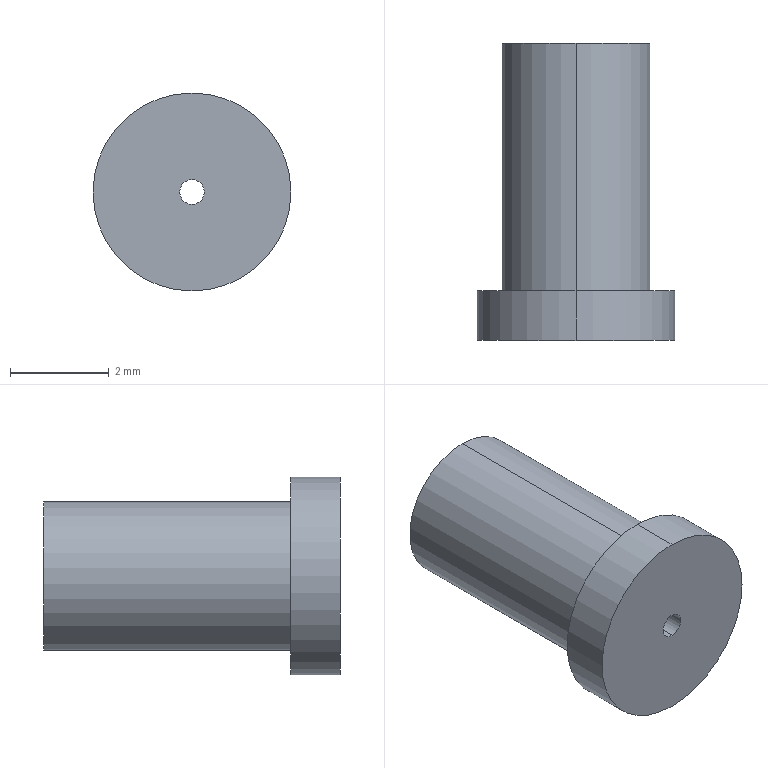Part | SolidWorks | features Revolution 1 | 1 solid | 9 faces | box 4 x 6 x 4 mm | volume 46.731 mm3 | cylinder 6 | plane 3 | commonest cylinder face diameters 0.5 x2 3 x2 4 x2
STEP:
#1=CARTESIAN_POINT('',(0.,3.773,-1.5));
#2=VERTEX_POINT('',#1);
#3=CARTESIAN_POINT('',(0.,3.773,1.5));
#4=VERTEX_POINT('',#3);
#5=CARTESIAN_POINT('',(0.,3.773,0.));
#6=DIRECTION('',(0.,-1.,0.));
#7=DIRECTION('',(0.,0.,-1.));
#8=AXIS2_PLACEMENT_3D('',#5,#6,#7);
#9=CIRCLE('',#8,1.5);
#10=EDGE_CURVE('',#2,#4,#9,.T.);
#11=ORIENTED_EDGE('',*,*,#10,.T.);
#12=CARTESIAN_POINT('',(0.,-1.227,1.5));
#13=VERTEX_POINT('',#12);
#14=CARTESIAN_POINT('',(0.,0.,1.5));
#15=DIRECTION('',(0.,-1.,0.));
#16=VECTOR('',#15,1000.);
#17=LINE('',#14,#16);
#18=EDGE_CURVE('',#4,#13,#17,.T.);
#19=ORIENTED_EDGE('',*,*,#18,.T.);
#20=CARTESIAN_POINT('',(0.,-1.227,-1.5));
#21=VERTEX_POINT('',#20);
#22=CARTESIAN_POINT('',(0.,-1.227,0.));
#23=DIRECTION('',(0.,-1.,0.));
#24=DIRECTION('',(0.,0.,-1.));
#25=AXIS2_PLACEMENT_3D('',#22,#23,#24);
#26=CIRCLE('',#25,1.5);
#27=EDGE_CURVE('',#21,#13,#26,.T.);
#28=ORIENTED_EDGE('',*,*,#27,.F.);
#29=CARTESIAN_POINT('',(0.,0.,-1.5));
#30=DIRECTION('',(0.,-1.,0.));
#31=VECTOR('',#30,1000.);
#32=LINE('',#29,#31);
#33=EDGE_CURVE('',#2,#21,#32,.T.);
#34=ORIENTED_EDGE('',*,*,#33,.F.);
#35=EDGE_LOOP('',(#11,#19,#28,#34));
#36=FACE_OUTER_BOUND('',#35,.T.);
#37=CARTESIAN_POINT('',(0.,0.,0.));
#38=DIRECTION('',(0.,-1.,0.));
#39=DIRECTION('',(0.,0.,-1.));
#40=AXIS2_PLACEMENT_3D('',#37,#38,#39);
#41=CYLINDRICAL_SURFACE('',#40,1.5);
#42=ADVANCED_FACE('',(#36),#41,.T.);
#43=CARTESIAN_POINT('',(0.,-1.227,-2.));
#44=VERTEX_POINT('',#43);
#45=CARTESIAN_POINT('',(0.,-1.227,2.));
#46=VERTEX_POINT('',#45);
#47=CARTESIAN_POINT('',(0.,-1.227,0.));
#48=DIRECTION('',(0.,-1.,0.));
#49=DIRECTION('',(0.,0.,-1.));
#50=AXIS2_PLACEMENT_3D('',#47,#48,#49);
#51=CIRCLE('',#50,2.);
#52=EDGE_CURVE('',#44,#46,#51,.T.);
#53=ORIENTED_EDGE('',*,*,#52,.T.);
#54=CARTESIAN_POINT('',(0.,-2.227,2.));
#55=VERTEX_POINT('',#54);
#56=CARTESIAN_POINT('',(0.,0.,2.));
#57=DIRECTION('',(0.,-1.,0.));
#58=VECTOR('',#57,1000.);
#59=LINE('',#56,#58);
#60=EDGE_CURVE('',#46,#55,#59,.T.);
#61=ORIENTED_EDGE('',*,*,#60,.T.);
#62=CARTESIAN_POINT('',(0.,-2.227,-2.));
#63=VERTEX_POINT('',#62);
#64=CARTESIAN_POINT('',(0.,-2.227,0.));
#65=DIRECTION('',(0.,-1.,0.));
#66=DIRECTION('',(0.,0.,-1.));
#67=AXIS2_PLACEMENT_3D('',#64,#65,#66);
#68=CIRCLE('',#67,2.);
#69=EDGE_CURVE('',#63,#55,#68,.T.);
#70=ORIENTED_EDGE('',*,*,#69,.F.);
#71=CARTESIAN_POINT('',(0.,0.,-2.));
#72=DIRECTION('',(0.,-1.,0.));
#73=VECTOR('',#72,1000.);
#74=LINE('',#71,#73);
#75=EDGE_CURVE('',#44,#63,#74,.T.);
#76=ORIENTED_EDGE('',*,*,#75,.F.);
#77=EDGE_LOOP('',(#53,#61,#70,#76));
#78=FACE_OUTER_BOUND('',#77,.T.);
#79=CARTESIAN_POINT('',(0.,0.,0.));
#80=DIRECTION('',(0.,-1.,0.));
#81=DIRECTION('',(0.,0.,-1.));
#82=AXIS2_PLACEMENT_3D('',#79,#80,#81);
#83=CYLINDRICAL_SURFACE('',#82,2.);
#84=ADVANCED_FACE('',(#78),#83,.T.);
#85=CARTESIAN_POINT('',(0.,3.773,0.25));
#86=VERTEX_POINT('',#85);
#87=CARTESIAN_POINT('',(0.,3.773,-0.25));
#88=VERTEX_POINT('',#87);
#89=CARTESIAN_POINT('',(0.,3.773,0.));
#90=DIRECTION('',(0.,-1.,0.));
#91=DIRECTION('',(0.,0.,-1.));
#92=AXIS2_PLACEMENT_3D('',#89,#90,#91);
#93=CIRCLE('',#92,0.25);
#94=EDGE_CURVE('',#86,#88,#93,.T.);
#95=ORIENTED_EDGE('',*,*,#94,.F.);
#96=CARTESIAN_POINT('',(0.,-2.227,0.25));
#97=VERTEX_POINT('',#96);
#98=CARTESIAN_POINT('',(0.,0.,0.25));
#99=DIRECTION('',(0.,-1.,0.));
#100=VECTOR('',#99,1000.);
#101=LINE('',#98,#100);
#102=EDGE_CURVE('',#86,#97,#101,.T.);
#103=ORIENTED_EDGE('',*,*,#102,.T.);
#104=CARTESIAN_POINT('',(0.,-2.227,-0.25));
#105=VERTEX_POINT('',#104);
#106=CARTESIAN_POINT('',(0.,-2.227,0.));
#107=DIRECTION('',(0.,-1.,0.));
#108=DIRECTION('',(0.,0.,-1.));
#109=AXIS2_PLACEMENT_3D('',#106,#107,#108);
#110=CIRCLE('',#109,0.25);
#111=EDGE_CURVE('',#97,#105,#110,.T.);
#112=ORIENTED_EDGE('',*,*,#111,.T.);
#113=CARTESIAN_POINT('',(0.,0.,-0.25));
#114=DIRECTION('',(0.,-1.,0.));
#115=VECTOR('',#114,1000.);
#116=LINE('',#113,#115);
#117=EDGE_CURVE('',#88,#105,#116,.T.);
#118=ORIENTED_EDGE('',*,*,#117,.F.);
#119=EDGE_LOOP('',(#95,#103,#112,#118));
#120=FACE_OUTER_BOUND('',#119,.T.);
#121=CARTESIAN_POINT('',(0.,0.,0.));
#122=DIRECTION('',(0.,-1.,0.));
#123=DIRECTION('',(0.,0.,-1.));
#124=AXIS2_PLACEMENT_3D('',#121,#122,#123);
#125=CYLINDRICAL_SURFACE('',#124,0.25);
#126=ADVANCED_FACE('',(#120),#125,.F.);
#127=CARTESIAN_POINT('',(0.,3.773,0.));
#128=DIRECTION('',(0.,-1.,0.));
#129=DIRECTION('',(0.,0.,-1.));
#130=AXIS2_PLACEMENT_3D('',#127,#128,#129);
#131=CIRCLE('',#130,0.25);
#132=EDGE_CURVE('',#88,#86,#131,.T.);
#133=ORIENTED_EDGE('',*,*,#132,.T.);
#134=ORIENTED_EDGE('',*,*,#94,.T.);
#135=EDGE_LOOP('',(#133,#134));
#136=FACE_BOUND('',#135,.T.);
#137=ORIENTED_EDGE('',*,*,#10,.F.);
#138=CARTESIAN_POINT('',(0.,3.773,0.));
#139=DIRECTION('',(0.,-1.,0.));
#140=DIRECTION('',(0.,0.,-1.));
#141=AXIS2_PLACEMENT_3D('',#138,#139,#140);
#142=CIRCLE('',#141,1.5);
#143=EDGE_CURVE('',#4,#2,#142,.T.);
#144=ORIENTED_EDGE('',*,*,#143,.F.);
#145=EDGE_LOOP('',(#137,#144));
#146=FACE_OUTER_BOUND('',#145,.T.);
#147=CARTESIAN_POINT('',(1.5,3.773,0.));
#148=DIRECTION('',(0.,1.,0.));
#149=DIRECTION('',(0.,0.,1.));
#150=AXIS2_PLACEMENT_3D('',#147,#148,#149);
#151=PLANE('',#150);
#152=ADVANCED_FACE('',(#136,#146),#151,.T.);
#153=ORIENTED_EDGE('',*,*,#102,.F.);
#154=ORIENTED_EDGE('',*,*,#132,.F.);
#155=ORIENTED_EDGE('',*,*,#117,.T.);
#156=CARTESIAN_POINT('',(0.,-2.227,0.));
#157=DIRECTION('',(0.,-1.,0.));
#158=DIRECTION('',(0.,0.,-1.));
#159=AXIS2_PLACEMENT_3D('',#156,#157,#158);
#160=CIRCLE('',#159,0.25);
#161=EDGE_CURVE('',#105,#97,#160,.T.);
#162=ORIENTED_EDGE('',*,*,#161,.T.);
#163=EDGE_LOOP('',(#153,#154,#155,#162));
#164=FACE_OUTER_BOUND('',#163,.T.);
#165=CARTESIAN_POINT('',(0.,0.,0.));
#166=DIRECTION('',(0.,-1.,0.));
#167=DIRECTION('',(0.,0.,-1.));
#168=AXIS2_PLACEMENT_3D('',#165,#166,#167);
#169=CYLINDRICAL_SURFACE('',#168,0.25);
#170=ADVANCED_FACE('',(#164),#169,.F.);
#171=ORIENTED_EDGE('',*,*,#69,.T.);
#172=CARTESIAN_POINT('',(0.,-2.227,0.));
#173=DIRECTION('',(0.,-1.,0.));
#174=DIRECTION('',(0.,0.,-1.));
#175=AXIS2_PLACEMENT_3D('',#172,#173,#174);
#176=CIRCLE('',#175,2.);
#177=EDGE_CURVE('',#55,#63,#176,.T.);
#178=ORIENTED_EDGE('',*,*,#177,.T.);
#179=EDGE_LOOP('',(#171,#178));
#180=FACE_OUTER_BOUND('',#179,.T.);
#181=ORIENTED_EDGE('',*,*,#161,.F.);
#182=ORIENTED_EDGE('',*,*,#111,.F.);
#183=EDGE_LOOP('',(#181,#182));
#184=FACE_BOUND('',#183,.T.);
#185=CARTESIAN_POINT('',(0.25,-2.227,0.));
#186=DIRECTION('',(0.,-1.,0.));
#187=DIRECTION('',(0.,0.,-1.));
#188=AXIS2_PLACEMENT_3D('',#185,#186,#187);
#189=PLANE('',#188);
#190=ADVANCED_FACE('',(#180,#184),#189,.T.);
#191=ORIENTED_EDGE('',*,*,#60,.F.);
#192=CARTESIAN_POINT('',(0.,-1.227,0.));
#193=DIRECTION('',(0.,-1.,0.));
#194=DIRECTION('',(0.,0.,-1.));
#195=AXIS2_PLACEMENT_3D('',#192,#193,#194);
#196=CIRCLE('',#195,2.);
#197=EDGE_CURVE('',#46,#44,#196,.T.);
#198=ORIENTED_EDGE('',*,*,#197,.T.);
#199=ORIENTED_EDGE('',*,*,#75,.T.);
#200=ORIENTED_EDGE('',*,*,#177,.F.);
#201=EDGE_LOOP('',(#191,#198,#199,#200));
#202=FACE_OUTER_BOUND('',#201,.T.);
#203=CARTESIAN_POINT('',(0.,0.,0.));
#204=DIRECTION('',(0.,-1.,0.));
#205=DIRECTION('',(0.,0.,-1.));
#206=AXIS2_PLACEMENT_3D('',#203,#204,#205);
#207=CYLINDRICAL_SURFACE('',#206,2.);
#208=ADVANCED_FACE('',(#202),#207,.T.);
#209=ORIENTED_EDGE('',*,*,#27,.T.);
#210=CARTESIAN_POINT('',(0.,-1.227,0.));
#211=DIRECTION('',(0.,-1.,0.));
#212=DIRECTION('',(0.,0.,-1.));
#213=AXIS2_PLACEMENT_3D('',#210,#211,#212);
#214=CIRCLE('',#213,1.5);
#215=EDGE_CURVE('',#13,#21,#214,.T.);
#216=ORIENTED_EDGE('',*,*,#215,.T.);
#217=EDGE_LOOP('',(#209,#216));
#218=FACE_BOUND('',#217,.T.);
#219=ORIENTED_EDGE('',*,*,#52,.F.);
#220=ORIENTED_EDGE('',*,*,#197,.F.);
#221=EDGE_LOOP('',(#219,#220));
#222=FACE_OUTER_BOUND('',#221,.T.);
#223=CARTESIAN_POINT('',(2.,-1.227,0.));
#224=DIRECTION('',(0.,1.,0.));
#225=DIRECTION('',(0.,0.,1.));
#226=AXIS2_PLACEMENT_3D('',#223,#224,#225);
#227=PLANE('',#226);
#228=ADVANCED_FACE('',(#218,#222),#227,.T.);
#229=ORIENTED_EDGE('',*,*,#18,.F.);
#230=ORIENTED_EDGE('',*,*,#143,.T.);
#231=ORIENTED_EDGE('',*,*,#33,.T.);
#232=ORIENTED_EDGE('',*,*,#215,.F.);
#233=EDGE_LOOP('',(#229,#230,#231,#232));
#234=FACE_OUTER_BOUND('',#233,.T.);
#235=CARTESIAN_POINT('',(0.,0.,0.));
#236=DIRECTION('',(0.,-1.,0.));
#237=DIRECTION('',(0.,0.,-1.));
#238=AXIS2_PLACEMENT_3D('',#235,#236,#237);
#239=CYLINDRICAL_SURFACE('',#238,1.5);
#240=ADVANCED_FACE('',(#234),#239,.T.);
#241=CLOSED_SHELL('',(#42,#84,#126,#152,#170,#190,#208,#228,#240));
#242=MANIFOLD_SOLID_BREP('',#241);
#243=CARTESIAN_POINT('',(0.,0.,0.));
#244=DIRECTION('',(0.,0.,1.));
#245=DIRECTION('',(1.,0.,0.));
#246=AXIS2_PLACEMENT_3D('',#243,#244,#245);
#247=(LENGTH_UNIT()NAMED_UNIT(*)SI_UNIT(.MILLI.,.METRE.));
#248=UNCERTAINTY_MEASURE_WITH_UNIT(LENGTH_MEASURE(0.00001),#247,'','');
#249=(NAMED_UNIT(*)PLANE_ANGLE_UNIT()SI_UNIT($,.RADIAN.));
#250=(NAMED_UNIT(*)SI_UNIT($,.STERADIAN.)SOLID_ANGLE_UNIT());
#251=(GEOMETRIC_REPRESENTATION_CONTEXT(3)GLOBAL_UNCERTAINTY_ASSIGNED_CONTEXT((#248))GLOBAL_UNIT_ASSIGNED_CONTEXT((#247,#249,#250))REPRESENTATION_CONTEXT('',''));
#252=ADVANCED_BREP_SHAPE_REPRESENTATION('',(#242,#246),#251);